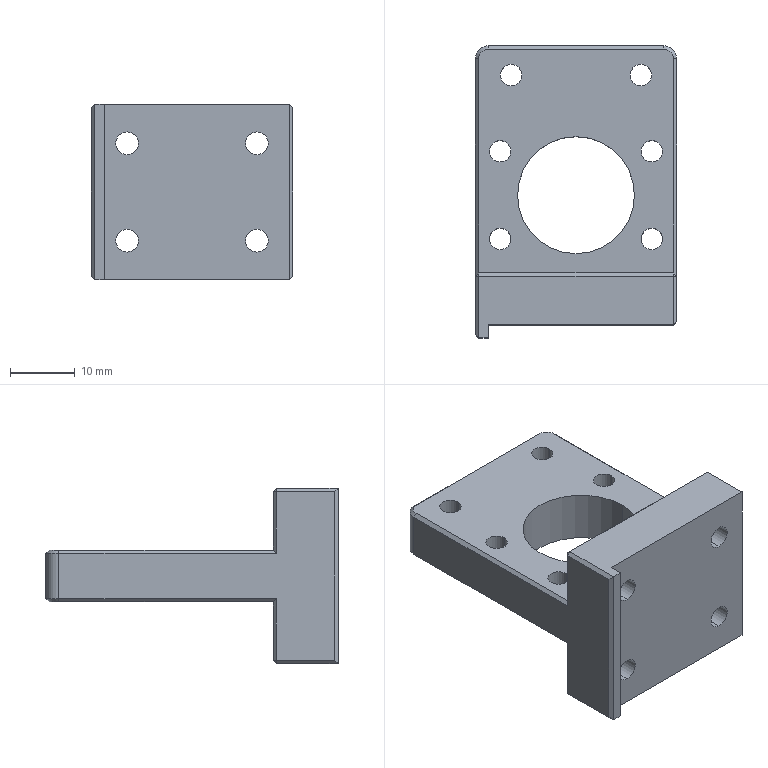Part | NX | features BREP 1 | 1 solid | 82 faces | box 31 x 45 x 27 mm | volume 12005 mm3 | plane 38 | cylinder 36 | cone 8 | commonest cylinder face diameters 3.3 x12 3.5 x8 7 x8 2.5 x4 4 x2 18 x2